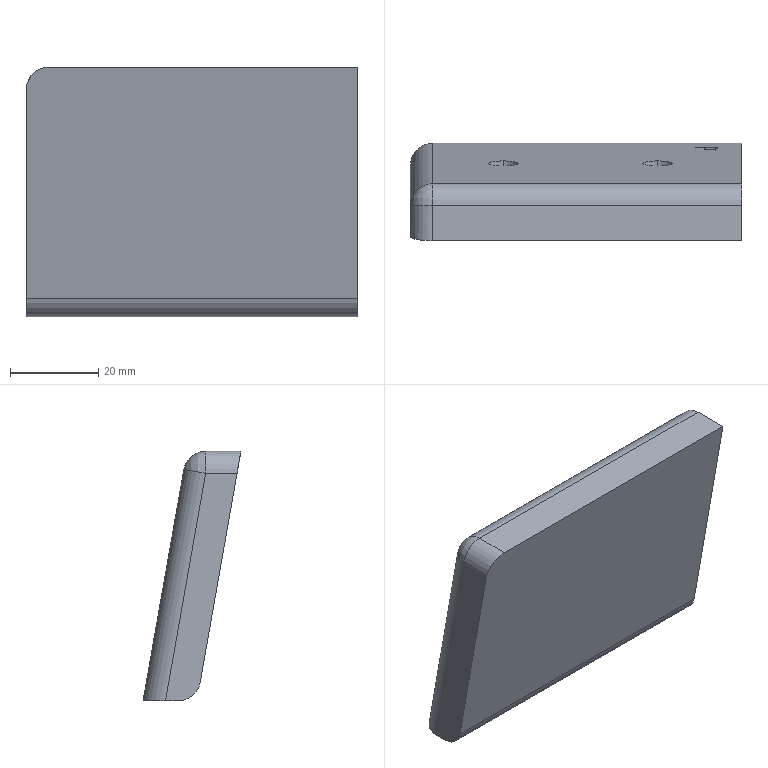Part | SolidWorks | features BaseBody 1 | 1 solid | 33 faces | box 75 x 22.148 x 56.5 mm | volume 50046 mm3 | plane 20 | cylinder 8 | cone 4 | sphere 1 | commonest cylinder face diameters 6.8 x4 10 x4
STEP:
#1=CARTESIAN_POINT('',(98.,284.297,22.336));
#2=VERTEX_POINT('',#1);
#3=CARTESIAN_POINT('',(98.,283.116,29.032));
#4=VERTEX_POINT('',#3);
#5=CARTESIAN_POINT('',(98.,283.707,25.684));
#6=DIRECTION('',(0.,0.9848,0.1736));
#7=DIRECTION('',(0.,0.1736,-0.9848));
#8=AXIS2_PLACEMENT_3D('',#5,#6,#7);
#9=CIRCLE('',#8,3.4);
#10=EDGE_CURVE('',#2,#4,#9,.T.);
#11=ORIENTED_EDGE('',*,*,#10,.T.);
#12=CARTESIAN_POINT('',(98.,274.253,27.47));
#13=VERTEX_POINT('',#12);
#14=CARTESIAN_POINT('',(98.,283.116,29.032));
#15=DIRECTION('',(0.,-0.9848,-0.1736));
#16=VECTOR('',#15,1000.);
#17=LINE('',#14,#16);
#18=EDGE_CURVE('',#4,#13,#17,.T.);
#19=ORIENTED_EDGE('',*,*,#18,.T.);
#20=CARTESIAN_POINT('',(98.,275.434,20.773));
#21=VERTEX_POINT('',#20);
#22=CARTESIAN_POINT('',(98.,274.843,24.121));
#23=DIRECTION('',(0.,0.9848,0.1736));
#24=DIRECTION('',(0.,0.1736,-0.9848));
#25=AXIS2_PLACEMENT_3D('',#22,#23,#24);
#26=CIRCLE('',#25,3.4);
#27=EDGE_CURVE('',#21,#13,#26,.T.);
#28=ORIENTED_EDGE('',*,*,#27,.F.);
#29=CARTESIAN_POINT('',(98.,284.297,22.336));
#30=DIRECTION('',(0.,-0.9848,-0.1736));
#31=VECTOR('',#30,1000.);
#32=LINE('',#29,#31);
#33=EDGE_CURVE('',#2,#21,#32,.T.);
#34=ORIENTED_EDGE('',*,*,#33,.F.);
#35=EDGE_LOOP('',(#11,#19,#28,#34));
#36=FACE_OUTER_BOUND('',#35,.T.);
#37=CARTESIAN_POINT('',(98.,283.707,25.684));
#38=DIRECTION('',(0.,-0.9848,-0.1736));
#39=DIRECTION('',(0.,0.1736,-0.9848));
#40=AXIS2_PLACEMENT_3D('',#37,#38,#39);
#41=CYLINDRICAL_SURFACE('',#40,3.4);
#42=ADVANCED_FACE('',(#36),#41,.F.);
#43=CARTESIAN_POINT('',(98.,272.831,23.767));
#44=VERTEX_POINT('',#43);
#45=CARTESIAN_POINT('',(98.,274.253,27.47));
#46=DIRECTION('',(0.,0.3584,0.9336));
#47=VECTOR('',#46,1000.);
#48=LINE('',#45,#47);
#49=EDGE_CURVE('',#44,#13,#48,.T.);
#50=ORIENTED_EDGE('',*,*,#49,.F.);
#51=CARTESIAN_POINT('',(98.,275.434,20.773));
#52=DIRECTION('',(0.,0.6561,-0.7547));
#53=VECTOR('',#52,1000.);
#54=LINE('',#51,#53);
#55=EDGE_CURVE('',#44,#21,#54,.T.);
#56=ORIENTED_EDGE('',*,*,#55,.T.);
#57=ORIENTED_EDGE('',*,*,#27,.T.);
#58=EDGE_LOOP('',(#50,#56,#57));
#59=FACE_OUTER_BOUND('',#58,.T.);
#60=CARTESIAN_POINT('',(98.,274.843,24.121));
#61=DIRECTION('',(0.,0.9848,0.1736));
#62=DIRECTION('',(0.,-0.1736,0.9848));
#63=AXIS2_PLACEMENT_3D('',#60,#61,#62);
#64=CONICAL_SURFACE('',#63,3.4,1.03);
#65=ADVANCED_FACE('',(#59),#64,.F.);
#66=CARTESIAN_POINT('',(133.,284.297,22.336));
#67=VERTEX_POINT('',#66);
#68=CARTESIAN_POINT('',(133.,283.116,29.032));
#69=VERTEX_POINT('',#68);
#70=CARTESIAN_POINT('',(133.,283.707,25.684));
#71=DIRECTION('',(0.,0.9848,0.1736));
#72=DIRECTION('',(0.,0.1736,-0.9848));
#73=AXIS2_PLACEMENT_3D('',#70,#71,#72);
#74=CIRCLE('',#73,3.4);
#75=EDGE_CURVE('',#67,#69,#74,.T.);
#76=ORIENTED_EDGE('',*,*,#75,.T.);
#77=CARTESIAN_POINT('',(133.,274.253,27.47));
#78=VERTEX_POINT('',#77);
#79=CARTESIAN_POINT('',(133.,283.116,29.032));
#80=DIRECTION('',(0.,-0.9848,-0.1736));
#81=VECTOR('',#80,1000.);
#82=LINE('',#79,#81);
#83=EDGE_CURVE('',#69,#78,#82,.T.);
#84=ORIENTED_EDGE('',*,*,#83,.T.);
#85=CARTESIAN_POINT('',(133.,275.434,20.773));
#86=VERTEX_POINT('',#85);
#87=CARTESIAN_POINT('',(133.,274.843,24.121));
#88=DIRECTION('',(0.,0.9848,0.1736));
#89=DIRECTION('',(0.,0.1736,-0.9848));
#90=AXIS2_PLACEMENT_3D('',#87,#88,#89);
#91=CIRCLE('',#90,3.4);
#92=EDGE_CURVE('',#86,#78,#91,.T.);
#93=ORIENTED_EDGE('',*,*,#92,.F.);
#94=CARTESIAN_POINT('',(133.,284.297,22.336));
#95=DIRECTION('',(0.,-0.9848,-0.1736));
#96=VECTOR('',#95,1000.);
#97=LINE('',#94,#96);
#98=EDGE_CURVE('',#67,#86,#97,.T.);
#99=ORIENTED_EDGE('',*,*,#98,.F.);
#100=EDGE_LOOP('',(#76,#84,#93,#99));
#101=FACE_OUTER_BOUND('',#100,.T.);
#102=CARTESIAN_POINT('',(133.,283.707,25.684));
#103=DIRECTION('',(0.,-0.9848,-0.1736));
#104=DIRECTION('',(0.,0.1736,-0.9848));
#105=AXIS2_PLACEMENT_3D('',#102,#103,#104);
#106=CYLINDRICAL_SURFACE('',#105,3.4);
#107=ADVANCED_FACE('',(#101),#106,.F.);
#108=CARTESIAN_POINT('',(133.,272.831,23.767));
#109=VERTEX_POINT('',#108);
#110=CARTESIAN_POINT('',(133.,274.253,27.47));
#111=DIRECTION('',(0.,0.3584,0.9336));
#112=VECTOR('',#111,1000.);
#113=LINE('',#110,#112);
#114=EDGE_CURVE('',#109,#78,#113,.T.);
#115=ORIENTED_EDGE('',*,*,#114,.F.);
#116=CARTESIAN_POINT('',(133.,275.434,20.773));
#117=DIRECTION('',(0.,0.6561,-0.7547));
#118=VECTOR('',#117,1000.);
#119=LINE('',#116,#118);
#120=EDGE_CURVE('',#109,#86,#119,.T.);
#121=ORIENTED_EDGE('',*,*,#120,.T.);
#122=ORIENTED_EDGE('',*,*,#92,.T.);
#123=EDGE_LOOP('',(#115,#121,#122));
#124=FACE_OUTER_BOUND('',#123,.T.);
#125=CARTESIAN_POINT('',(133.,274.843,24.121));
#126=DIRECTION('',(0.,0.9848,0.1736));
#127=DIRECTION('',(0.,-0.1736,0.9848));
#128=AXIS2_PLACEMENT_3D('',#125,#126,#127);
#129=CONICAL_SURFACE('',#128,3.4,1.03);
#130=ADVANCED_FACE('',(#124),#129,.F.);
#131=CARTESIAN_POINT('',(77.,267.058,51.));
#132=VERTEX_POINT('',#131);
#133=CARTESIAN_POINT('',(77.,275.41,3.632));
#134=VERTEX_POINT('',#133);
#135=CARTESIAN_POINT('',(77.,270.574,31.056));
#136=DIRECTION('',(0.,0.1736,-0.9848));
#137=VECTOR('',#136,1000.);
#138=LINE('',#135,#137);
#139=EDGE_CURVE('',#132,#134,#138,.T.);
#140=ORIENTED_EDGE('',*,*,#139,.T.);
#141=CARTESIAN_POINT('',(152.,275.41,3.632));
#142=VERTEX_POINT('',#141);
#143=CARTESIAN_POINT('',(-4.,275.41,3.632));
#144=DIRECTION('',(-1.,0.,0.));
#145=VECTOR('',#144,1000.);
#146=LINE('',#143,#145);
#147=EDGE_CURVE('',#142,#134,#146,.T.);
#148=ORIENTED_EDGE('',*,*,#147,.F.);
#149=CARTESIAN_POINT('',(152.,266.176,56.));
#150=VERTEX_POINT('',#149);
#151=CARTESIAN_POINT('',(152.,271.705,24.642));
#152=DIRECTION('',(0.,0.1736,-0.9848));
#153=VECTOR('',#152,1000.);
#154=LINE('',#151,#153);
#155=EDGE_CURVE('',#150,#142,#154,.T.);
#156=ORIENTED_EDGE('',*,*,#155,.F.);
#157=CARTESIAN_POINT('',(82.,266.176,56.));
#158=VERTEX_POINT('',#157);
#159=CARTESIAN_POINT('',(-4.,266.176,56.));
#160=DIRECTION('',(-1.,0.,0.));
#161=VECTOR('',#160,1000.);
#162=LINE('',#159,#161);
#163=EDGE_CURVE('',#150,#158,#162,.T.);
#164=ORIENTED_EDGE('',*,*,#163,.T.);
#165=CARTESIAN_POINT('',(77.,267.058,51.));
#166=CARTESIAN_POINT('',(77.,266.541,53.929));
#167=CARTESIAN_POINT('',(79.071,266.176,56.));
#168=CARTESIAN_POINT('',(82.,266.176,56.));
#169=(BOUNDED_CURVE()B_SPLINE_CURVE(3,(#165,#166,#167,#168),.UNSPECIFIED.,.F.,.T.)B_SPLINE_CURVE_WITH_KNOTS((4,4),(4.712,6.283),.UNSPECIFIED.)CURVE()GEOMETRIC_REPRESENTATION_ITEM()RATIONAL_B_SPLINE_CURVE((1.,0.8047,0.8047,1.))REPRESENTATION_ITEM(''));
#170=EDGE_CURVE('',#132,#158,#169,.T.);
#171=ORIENTED_EDGE('',*,*,#170,.F.);
#172=EDGE_LOOP('',(#140,#148,#156,#164,#171));
#173=FACE_OUTER_BOUND('',#172,.T.);
#174=CARTESIAN_POINT('',(-4.,266.352,55.));
#175=DIRECTION('',(0.,0.9848,0.1736));
#176=DIRECTION('',(0.,-0.1736,0.9848));
#177=AXIS2_PLACEMENT_3D('',#174,#175,#176);
#178=PLANE('',#177);
#179=ADVANCED_FACE('',(#173),#178,.F.);
#180=CARTESIAN_POINT('',(146.015,286.85,7.856));
#181=VERTEX_POINT('',#180);
#182=CARTESIAN_POINT('',(146.015,286.503,9.826));
#183=VERTEX_POINT('',#182);
#184=CARTESIAN_POINT('',(146.015,286.85,7.856));
#185=DIRECTION('',(0.,-0.1736,0.9848));
#186=VECTOR('',#185,1000.);
#187=LINE('',#184,#186);
#188=EDGE_CURVE('',#181,#183,#187,.T.);
#189=ORIENTED_EDGE('',*,*,#188,.F.);
#190=CARTESIAN_POINT('',(143.515,286.85,7.856));
#191=VERTEX_POINT('',#190);
#192=CARTESIAN_POINT('',(146.015,286.85,7.856));
#193=DIRECTION('',(-1.,0.,0.));
#194=VECTOR('',#193,1000.);
#195=LINE('',#192,#194);
#196=EDGE_CURVE('',#181,#191,#195,.T.);
#197=ORIENTED_EDGE('',*,*,#196,.T.);
#198=CARTESIAN_POINT('',(143.515,287.284,5.394));
#199=VERTEX_POINT('',#198);
#200=CARTESIAN_POINT('',(143.515,287.284,5.394));
#201=DIRECTION('',(0.,-0.1736,0.9848));
#202=VECTOR('',#201,1000.);
#203=LINE('',#200,#202);
#204=EDGE_CURVE('',#199,#191,#203,.T.);
#205=ORIENTED_EDGE('',*,*,#204,.F.);
#206=CARTESIAN_POINT('',(141.515,287.284,5.394));
#207=VERTEX_POINT('',#206);
#208=CARTESIAN_POINT('',(143.515,287.284,5.394));
#209=DIRECTION('',(-1.,0.,0.));
#210=VECTOR('',#209,1000.);
#211=LINE('',#208,#210);
#212=EDGE_CURVE('',#199,#207,#211,.T.);
#213=ORIENTED_EDGE('',*,*,#212,.T.);
#214=CARTESIAN_POINT('',(141.515,287.371,4.902));
#215=VERTEX_POINT('',#214);
#216=CARTESIAN_POINT('',(141.515,287.284,5.394));
#217=DIRECTION('',(0.,0.1736,-0.9848));
#218=VECTOR('',#217,1000.);
#219=LINE('',#216,#218);
#220=EDGE_CURVE('',#207,#215,#219,.T.);
#221=ORIENTED_EDGE('',*,*,#220,.T.);
#222=CARTESIAN_POINT('',(146.515,287.371,4.902));
#223=VERTEX_POINT('',#222);
#224=CARTESIAN_POINT('',(146.515,287.371,4.902));
#225=DIRECTION('',(-1.,0.,0.));
#226=VECTOR('',#225,1000.);
#227=LINE('',#224,#226);
#228=EDGE_CURVE('',#223,#215,#227,.T.);
#229=ORIENTED_EDGE('',*,*,#228,.F.);
#230=CARTESIAN_POINT('',(146.515,286.503,9.826));
#231=VERTEX_POINT('',#230);
#232=CARTESIAN_POINT('',(146.515,287.371,4.902));
#233=DIRECTION('',(0.,-0.1736,0.9848));
#234=VECTOR('',#233,1000.);
#235=LINE('',#232,#234);
#236=EDGE_CURVE('',#223,#231,#235,.T.);
#237=ORIENTED_EDGE('',*,*,#236,.T.);
#238=CARTESIAN_POINT('',(146.515,286.503,9.826));
#239=DIRECTION('',(-1.,0.,0.));
#240=VECTOR('',#239,1000.);
#241=LINE('',#238,#240);
#242=EDGE_CURVE('',#231,#183,#241,.T.);
#243=ORIENTED_EDGE('',*,*,#242,.T.);
#244=EDGE_LOOP('',(#189,#197,#205,#213,#221,#229,#237,#243));
#245=FACE_BOUND('',#244,.T.);
#246=ORIENTED_EDGE('',*,*,#75,.F.);
#247=CARTESIAN_POINT('',(133.,283.707,25.684));
#248=DIRECTION('',(0.,0.9848,0.1736));
#249=DIRECTION('',(0.,0.1736,-0.9848));
#250=AXIS2_PLACEMENT_3D('',#247,#248,#249);
#251=CIRCLE('',#250,3.4);
#252=EDGE_CURVE('',#69,#67,#251,.T.);
#253=ORIENTED_EDGE('',*,*,#252,.F.);
#254=EDGE_LOOP('',(#246,#253));
#255=FACE_BOUND('',#254,.T.);
#256=ORIENTED_EDGE('',*,*,#10,.F.);
#257=CARTESIAN_POINT('',(98.,283.707,25.684));
#258=DIRECTION('',(0.,0.9848,0.1736));
#259=DIRECTION('',(0.,0.1736,-0.9848));
#260=AXIS2_PLACEMENT_3D('',#257,#258,#259);
#261=CIRCLE('',#260,3.4);
#262=EDGE_CURVE('',#4,#2,#261,.T.);
#263=ORIENTED_EDGE('',*,*,#262,.F.);
#264=EDGE_LOOP('',(#256,#263));
#265=FACE_BOUND('',#264,.T.);
#266=CARTESIAN_POINT('',(82.,279.09,51.868));
#267=VERTEX_POINT('',#266);
#268=CARTESIAN_POINT('',(152.,279.09,51.868));
#269=VERTEX_POINT('',#268);
#270=CARTESIAN_POINT('',(188.,279.09,51.868));
#271=DIRECTION('',(1.,0.,0.));
#272=VECTOR('',#271,1000.);
#273=LINE('',#270,#272);
#274=EDGE_CURVE('',#267,#269,#273,.T.);
#275=ORIENTED_EDGE('',*,*,#274,.T.);
#276=CARTESIAN_POINT('',(152.,288.324,-0.5));
#277=VERTEX_POINT('',#276);
#278=CARTESIAN_POINT('',(152.,283.523,26.726));
#279=DIRECTION('',(0.,0.1736,-0.9848));
#280=VECTOR('',#279,1000.);
#281=LINE('',#278,#280);
#282=EDGE_CURVE('',#269,#277,#281,.T.);
#283=ORIENTED_EDGE('',*,*,#282,.T.);
#284=CARTESIAN_POINT('',(82.,288.324,-0.5));
#285=VERTEX_POINT('',#284);
#286=CARTESIAN_POINT('',(-429.,288.324,-0.5));
#287=DIRECTION('',(1.,0.,0.));
#288=VECTOR('',#287,1000.);
#289=LINE('',#286,#288);
#290=EDGE_CURVE('',#285,#277,#289,.T.);
#291=ORIENTED_EDGE('',*,*,#290,.F.);
#292=CARTESIAN_POINT('',(82.,288.324,-0.5));
#293=DIRECTION('',(0.,0.1736,-0.9848));
#294=VECTOR('',#293,1000.);
#295=LINE('',#292,#294);
#296=EDGE_CURVE('',#267,#285,#295,.T.);
#297=ORIENTED_EDGE('',*,*,#296,.F.);
#298=EDGE_LOOP('',(#275,#283,#291,#297));
#299=FACE_OUTER_BOUND('',#298,.T.);
#300=CARTESIAN_POINT('',(140.5,282.887,30.334));
#301=DIRECTION('',(0.,-0.9848,-0.1736));
#302=DIRECTION('',(0.,0.1736,-0.9848));
#303=AXIS2_PLACEMENT_3D('',#300,#301,#302);
#304=PLANE('',#303);
#305=ADVANCED_FACE('',(#245,#255,#265,#299),#304,.F.);
#306=ORIENTED_EDGE('',*,*,#163,.F.);
#307=CARTESIAN_POINT('',(152.,274.166,56.));
#308=VERTEX_POINT('',#307);
#309=CARTESIAN_POINT('',(152.,275.152,56.));
#310=DIRECTION('',(0.,1.,0.));
#311=VECTOR('',#310,1000.);
#312=LINE('',#309,#311);
#313=EDGE_CURVE('',#150,#308,#312,.T.);
#314=ORIENTED_EDGE('',*,*,#313,.T.);
#315=CARTESIAN_POINT('',(82.,274.166,56.));
#316=VERTEX_POINT('',#315);
#317=CARTESIAN_POINT('',(93.,274.166,56.));
#318=DIRECTION('',(-1.,0.,0.));
#319=VECTOR('',#318,1000.);
#320=LINE('',#317,#319);
#321=EDGE_CURVE('',#308,#316,#320,.T.);
#322=ORIENTED_EDGE('',*,*,#321,.T.);
#323=CARTESIAN_POINT('',(82.,274.166,56.));
#324=DIRECTION('',(0.,1.,0.));
#325=VECTOR('',#324,1000.);
#326=LINE('',#323,#325);
#327=EDGE_CURVE('',#158,#316,#326,.T.);
#328=ORIENTED_EDGE('',*,*,#327,.F.);
#329=EDGE_LOOP('',(#306,#314,#322,#328));
#330=FACE_OUTER_BOUND('',#329,.T.);
#331=CARTESIAN_POINT('',(138.,235.588,56.));
#332=DIRECTION('',(0.,0.,-1.));
#333=DIRECTION('',(1.,0.,0.));
#334=AXIS2_PLACEMENT_3D('',#331,#332,#333);
#335=PLANE('',#334);
#336=ADVANCED_FACE('',(#330),#335,.F.);
#337=ORIENTED_EDGE('',*,*,#290,.T.);
#338=CARTESIAN_POINT('',(152.,280.334,-0.5));
#339=VERTEX_POINT('',#338);
#340=CARTESIAN_POINT('',(152.,275.152,-0.5));
#341=DIRECTION('',(0.,1.,0.));
#342=VECTOR('',#341,1000.);
#343=LINE('',#340,#342);
#344=EDGE_CURVE('',#339,#277,#343,.T.);
#345=ORIENTED_EDGE('',*,*,#344,.F.);
#346=CARTESIAN_POINT('',(77.,280.334,-0.5));
#347=VERTEX_POINT('',#346);
#348=CARTESIAN_POINT('',(-429.,280.334,-0.5));
#349=DIRECTION('',(1.,0.,0.));
#350=VECTOR('',#349,1000.);
#351=LINE('',#348,#350);
#352=EDGE_CURVE('',#347,#339,#351,.T.);
#353=ORIENTED_EDGE('',*,*,#352,.F.);
#354=CARTESIAN_POINT('',(77.,283.246,-0.5));
#355=VERTEX_POINT('',#354);
#356=CARTESIAN_POINT('',(77.,355.,-0.5));
#357=DIRECTION('',(0.,-1.,0.));
#358=VECTOR('',#357,1000.);
#359=LINE('',#356,#358);
#360=EDGE_CURVE('',#355,#347,#359,.T.);
#361=ORIENTED_EDGE('',*,*,#360,.F.);
#362=CARTESIAN_POINT('',(82.,288.324,-0.5));
#363=CARTESIAN_POINT('',(79.071,288.324,-0.5));
#364=CARTESIAN_POINT('',(77.,286.221,-0.5));
#365=CARTESIAN_POINT('',(77.,283.246,-0.5));
#366=(BOUNDED_CURVE()B_SPLINE_CURVE(3,(#362,#363,#364,#365),.UNSPECIFIED.,.F.,.T.)B_SPLINE_CURVE_WITH_KNOTS((4,4),(0.,1.571),.UNSPECIFIED.)CURVE()GEOMETRIC_REPRESENTATION_ITEM()RATIONAL_B_SPLINE_CURVE((1.,0.8047,0.8047,1.))REPRESENTATION_ITEM(''));
#367=EDGE_CURVE('',#285,#355,#366,.T.);
#368=ORIENTED_EDGE('',*,*,#367,.F.);
#369=EDGE_LOOP('',(#337,#345,#353,#361,#368));
#370=FACE_OUTER_BOUND('',#369,.T.);
#371=CARTESIAN_POINT('',(-429.,355.,-0.5));
#372=DIRECTION('',(0.,0.,-1.));
#373=DIRECTION('',(1.,0.,0.));
#374=AXIS2_PLACEMENT_3D('',#371,#372,#373);
#375=PLANE('',#374);
#376=ADVANCED_FACE('',(#370),#375,.T.);
#377=ORIENTED_EDGE('',*,*,#321,.F.);
#378=CARTESIAN_POINT('',(152.,274.166,51.));
#379=DIRECTION('',(1.,0.,0.));
#380=DIRECTION('',(0.,0.,-1.));
#381=AXIS2_PLACEMENT_3D('',#378,#379,#380);
#382=CIRCLE('',#381,5.);
#383=EDGE_CURVE('',#269,#308,#382,.T.);
#384=ORIENTED_EDGE('',*,*,#383,.F.);
#385=ORIENTED_EDGE('',*,*,#274,.F.);
#386=CARTESIAN_POINT('',(82.,274.166,51.));
#387=DIRECTION('',(-1.,0.,0.));
#388=DIRECTION('',(0.,1.,0.));
#389=AXIS2_PLACEMENT_3D('',#386,#387,#388);
#390=CIRCLE('',#389,5.);
#391=EDGE_CURVE('',#316,#267,#390,.T.);
#392=ORIENTED_EDGE('',*,*,#391,.F.);
#393=EDGE_LOOP('',(#377,#384,#385,#392));
#394=FACE_OUTER_BOUND('',#393,.T.);
#395=CARTESIAN_POINT('',(140.5,274.166,51.));
#396=DIRECTION('',(-1.,0.,0.));
#397=DIRECTION('',(0.,1.,0.));
#398=AXIS2_PLACEMENT_3D('',#395,#396,#397);
#399=CYLINDRICAL_SURFACE('',#398,5.);
#400=ADVANCED_FACE('',(#394),#399,.T.);
#401=ORIENTED_EDGE('',*,*,#147,.T.);
#402=CARTESIAN_POINT('',(77.,280.334,4.5));
#403=DIRECTION('',(1.,0.,0.));
#404=DIRECTION('',(0.,0.,-1.));
#405=AXIS2_PLACEMENT_3D('',#402,#403,#404);
#406=CIRCLE('',#405,5.);
#407=EDGE_CURVE('',#134,#347,#406,.T.);
#408=ORIENTED_EDGE('',*,*,#407,.T.);
#409=ORIENTED_EDGE('',*,*,#352,.T.);
#410=CARTESIAN_POINT('',(152.,280.334,4.5));
#411=DIRECTION('',(1.,0.,0.));
#412=DIRECTION('',(0.,0.,-1.));
#413=AXIS2_PLACEMENT_3D('',#410,#411,#412);
#414=CIRCLE('',#413,5.);
#415=EDGE_CURVE('',#142,#339,#414,.T.);
#416=ORIENTED_EDGE('',*,*,#415,.F.);
#417=EDGE_LOOP('',(#401,#408,#409,#416));
#418=FACE_OUTER_BOUND('',#417,.T.);
#419=CARTESIAN_POINT('',(-4.,280.334,4.5));
#420=DIRECTION('',(1.,0.,0.));
#421=DIRECTION('',(0.,-1.,0.));
#422=AXIS2_PLACEMENT_3D('',#419,#420,#421);
#423=CYLINDRICAL_SURFACE('',#422,5.);
#424=ADVANCED_FACE('',(#418),#423,.T.);
#425=CARTESIAN_POINT('',(77.,274.166,51.));
#426=VERTEX_POINT('',#425);
#427=CARTESIAN_POINT('',(77.,274.166,51.));
#428=DIRECTION('',(0.,-0.1736,0.9848));
#429=VECTOR('',#428,1000.);
#430=LINE('',#427,#429);
#431=EDGE_CURVE('',#355,#426,#430,.T.);
#432=ORIENTED_EDGE('',*,*,#431,.F.);
#433=ORIENTED_EDGE('',*,*,#360,.T.);
#434=ORIENTED_EDGE('',*,*,#407,.F.);
#435=ORIENTED_EDGE('',*,*,#139,.F.);
#436=CARTESIAN_POINT('',(77.,266.176,51.));
#437=DIRECTION('',(0.,-1.,0.));
#438=VECTOR('',#437,1000.);
#439=LINE('',#436,#438);
#440=EDGE_CURVE('',#426,#132,#439,.T.);
#441=ORIENTED_EDGE('',*,*,#440,.F.);
#442=EDGE_LOOP('',(#432,#433,#434,#435,#441));
#443=FACE_OUTER_BOUND('',#442,.T.);
#444=CARTESIAN_POINT('',(77.,240.481,25.75));
#445=DIRECTION('',(-1.,0.,0.));
#446=DIRECTION('',(0.,0.,-1.));
#447=AXIS2_PLACEMENT_3D('',#444,#445,#446);
#448=PLANE('',#447);
#449=ADVANCED_FACE('',(#443),#448,.T.);
#450=ORIENTED_EDGE('',*,*,#120,.F.);
#451=ORIENTED_EDGE('',*,*,#114,.T.);
#452=CARTESIAN_POINT('',(133.,274.843,24.121));
#453=DIRECTION('',(0.,0.9848,0.1736));
#454=DIRECTION('',(0.,0.1736,-0.9848));
#455=AXIS2_PLACEMENT_3D('',#452,#453,#454);
#456=CIRCLE('',#455,3.4);
#457=EDGE_CURVE('',#78,#86,#456,.T.);
#458=ORIENTED_EDGE('',*,*,#457,.T.);
#459=EDGE_LOOP('',(#450,#451,#458));
#460=FACE_OUTER_BOUND('',#459,.T.);
#461=CARTESIAN_POINT('',(133.,274.843,24.121));
#462=DIRECTION('',(0.,0.9848,0.1736));
#463=DIRECTION('',(0.,-0.1736,0.9848));
#464=AXIS2_PLACEMENT_3D('',#461,#462,#463);
#465=CONICAL_SURFACE('',#464,3.4,1.03);
#466=ADVANCED_FACE('',(#460),#465,.F.);
#467=ORIENTED_EDGE('',*,*,#83,.F.);
#468=ORIENTED_EDGE('',*,*,#252,.T.);
#469=ORIENTED_EDGE('',*,*,#98,.T.);
#470=ORIENTED_EDGE('',*,*,#457,.F.);
#471=EDGE_LOOP('',(#467,#468,#469,#470));
#472=FACE_OUTER_BOUND('',#471,.T.);
#473=CARTESIAN_POINT('',(133.,283.707,25.684));
#474=DIRECTION('',(0.,-0.9848,-0.1736));
#475=DIRECTION('',(0.,0.1736,-0.9848));
#476=AXIS2_PLACEMENT_3D('',#473,#474,#475);
#477=CYLINDRICAL_SURFACE('',#476,3.4);
#478=ADVANCED_FACE('',(#472),#477,.F.);
#479=ORIENTED_EDGE('',*,*,#55,.F.);
#480=ORIENTED_EDGE('',*,*,#49,.T.);
#481=CARTESIAN_POINT('',(98.,274.843,24.121));
#482=DIRECTION('',(0.,0.9848,0.1736));
#483=DIRECTION('',(0.,0.1736,-0.9848));
#484=AXIS2_PLACEMENT_3D('',#481,#482,#483);
#485=CIRCLE('',#484,3.4);
#486=EDGE_CURVE('',#13,#21,#485,.T.);
#487=ORIENTED_EDGE('',*,*,#486,.T.);
#488=EDGE_LOOP('',(#479,#480,#487));
#489=FACE_OUTER_BOUND('',#488,.T.);
#490=CARTESIAN_POINT('',(98.,274.843,24.121));
#491=DIRECTION('',(0.,0.9848,0.1736));
#492=DIRECTION('',(0.,-0.1736,0.9848));
#493=AXIS2_PLACEMENT_3D('',#490,#491,#492);
#494=CONICAL_SURFACE('',#493,3.4,1.03);
#495=ADVANCED_FACE('',(#489),#494,.F.);
#496=ORIENTED_EDGE('',*,*,#18,.F.);
#497=ORIENTED_EDGE('',*,*,#262,.T.);
#498=ORIENTED_EDGE('',*,*,#33,.T.);
#499=ORIENTED_EDGE('',*,*,#486,.F.);
#500=EDGE_LOOP('',(#496,#497,#498,#499));
#501=FACE_OUTER_BOUND('',#500,.T.);
#502=CARTESIAN_POINT('',(98.,283.707,25.684));
#503=DIRECTION('',(0.,-0.9848,-0.1736));
#504=DIRECTION('',(0.,0.1736,-0.9848));
#505=AXIS2_PLACEMENT_3D('',#502,#503,#504);
#506=CYLINDRICAL_SURFACE('',#505,3.4);
#507=ADVANCED_FACE('',(#501),#506,.F.);
#508=ORIENTED_EDGE('',*,*,#155,.T.);
#509=ORIENTED_EDGE('',*,*,#415,.T.);
#510=ORIENTED_EDGE('',*,*,#344,.T.);
#511=ORIENTED_EDGE('',*,*,#282,.F.);
#512=ORIENTED_EDGE('',*,*,#383,.T.);
#513=ORIENTED_EDGE('',*,*,#313,.F.);
#514=EDGE_LOOP('',(#508,#509,#510,#511,#512,#513));
#515=FACE_OUTER_BOUND('',#514,.T.);
#516=CARTESIAN_POINT('',(152.,275.152,25.25));
#517=DIRECTION('',(1.,0.,0.));
#518=DIRECTION('',(0.,0.,1.));
#519=AXIS2_PLACEMENT_3D('',#516,#517,#518);
#520=PLANE('',#519);
#521=ADVANCED_FACE('',(#515),#520,.T.);
#522=ORIENTED_EDGE('',*,*,#367,.T.);
#523=ORIENTED_EDGE('',*,*,#431,.T.);
#524=CARTESIAN_POINT('',(82.,274.166,51.));
#525=DIRECTION('',(0.,0.1736,-0.9848));
#526=DIRECTION('',(0.,-0.9848,-0.1736));
#527=AXIS2_PLACEMENT_3D('',#524,#525,#526);
#528=CIRCLE('',#527,5.);
#529=EDGE_CURVE('',#426,#267,#528,.T.);
#530=ORIENTED_EDGE('',*,*,#529,.T.);
#531=ORIENTED_EDGE('',*,*,#296,.T.);
#532=EDGE_LOOP('',(#522,#523,#530,#531));
#533=FACE_OUTER_BOUND('',#532,.T.);
#534=CARTESIAN_POINT('',(82.,277.468,32.272));
#535=DIRECTION('',(0.,0.1736,-0.9848));
#536=DIRECTION('',(0.,0.9848,0.1736));
#537=AXIS2_PLACEMENT_3D('',#534,#535,#536);
#538=CYLINDRICAL_SURFACE('',#537,5.);
#539=ADVANCED_FACE('',(#533),#538,.T.);
#540=ORIENTED_EDGE('',*,*,#529,.F.);
#541=CARTESIAN_POINT('',(82.,274.166,51.));
#542=DIRECTION('',(0.,1.,0.));
#543=DIRECTION('',(0.,0.,-1.));
#544=AXIS2_PLACEMENT_3D('',#541,#542,#543);
#545=CIRCLE('',#544,5.);
#546=EDGE_CURVE('',#426,#316,#545,.T.);
#547=ORIENTED_EDGE('',*,*,#546,.T.);
#548=ORIENTED_EDGE('',*,*,#391,.T.);
#549=EDGE_LOOP('',(#540,#547,#548));
#550=FACE_OUTER_BOUND('',#549,.T.);
#551=CARTESIAN_POINT('',(82.,274.166,51.));
#552=DIRECTION('',(0.,-1.,0.));
#553=DIRECTION('',(-1.,0.,0.));
#554=AXIS2_PLACEMENT_3D('',#551,#552,#553);
#555=SPHERICAL_SURFACE('',#554,5.);
#556=ADVANCED_FACE('',(#550),#555,.T.);
#557=ORIENTED_EDGE('',*,*,#170,.T.);
#558=ORIENTED_EDGE('',*,*,#327,.T.);
#559=ORIENTED_EDGE('',*,*,#546,.F.);
#560=ORIENTED_EDGE('',*,*,#440,.T.);
#561=EDGE_LOOP('',(#557,#558,#559,#560));
#562=FACE_OUTER_BOUND('',#561,.T.);
#563=CARTESIAN_POINT('',(82.,235.588,51.));
#564=DIRECTION('',(0.,-1.,0.));
#565=DIRECTION('',(0.,0.,-1.));
#566=AXIS2_PLACEMENT_3D('',#563,#564,#565);
#567=CYLINDRICAL_SURFACE('',#566,5.);
#568=ADVANCED_FACE('',(#562),#567,.T.);
#569=CARTESIAN_POINT('',(146.015,287.038,5.351));
#570=VERTEX_POINT('',#569);
#571=CARTESIAN_POINT('',(146.015,286.691,7.32));
#572=VERTEX_POINT('',#571);
#573=CARTESIAN_POINT('',(146.015,287.038,5.351));
#574=DIRECTION('',(0.,-0.1736,0.9848));
#575=VECTOR('',#574,1000.);
#576=LINE('',#573,#575);
#577=EDGE_CURVE('',#570,#572,#576,.T.);
#578=ORIENTED_EDGE('',*,*,#577,.F.);
#579=CARTESIAN_POINT('',(146.015,287.284,5.394));
#580=VERTEX_POINT('',#579);
#581=CARTESIAN_POINT('',(146.015,287.284,5.394));
#582=DIRECTION('',(0.,-0.9848,-0.1736));
#583=VECTOR('',#582,1000.);
#584=LINE('',#581,#583);
#585=EDGE_CURVE('',#580,#570,#584,.T.);
#586=ORIENTED_EDGE('',*,*,#585,.F.);
#587=CARTESIAN_POINT('',(146.015,286.937,7.364));
#588=VERTEX_POINT('',#587);
#589=CARTESIAN_POINT('',(146.015,287.284,5.394));
#590=DIRECTION('',(0.,-0.1736,0.9848));
#591=VECTOR('',#590,1000.);
#592=LINE('',#589,#591);
#593=EDGE_CURVE('',#580,#588,#592,.T.);
#594=ORIENTED_EDGE('',*,*,#593,.T.);
#595=CARTESIAN_POINT('',(146.015,286.937,7.364));
#596=DIRECTION('',(0.,-0.9848,-0.1736));
#597=VECTOR('',#596,1000.);
#598=LINE('',#595,#597);
#599=EDGE_CURVE('',#588,#572,#598,.T.);
#600=ORIENTED_EDGE('',*,*,#599,.T.);
#601=EDGE_LOOP('',(#578,#586,#594,#600));
#602=FACE_OUTER_BOUND('',#601,.T.);
#603=CARTESIAN_POINT('',(146.015,287.284,5.394));
#604=DIRECTION('',(1.,0.,0.));
#605=DIRECTION('',(0.,0.9848,0.1736));
#606=AXIS2_PLACEMENT_3D('',#603,#604,#605);
#607=PLANE('',#606);
#608=ADVANCED_FACE('',(#602),#607,.T.);
#609=CARTESIAN_POINT('',(144.015,287.038,5.351));
#610=VERTEX_POINT('',#609);
#611=CARTESIAN_POINT('',(146.015,287.038,5.351));
#612=DIRECTION('',(-1.,0.,0.));
#613=VECTOR('',#612,1000.);
#614=LINE('',#611,#613);
#615=EDGE_CURVE('',#570,#610,#614,.T.);
#616=ORIENTED_EDGE('',*,*,#615,.T.);
#617=CARTESIAN_POINT('',(144.015,287.284,5.394));
#618=VERTEX_POINT('',#617);
#619=CARTESIAN_POINT('',(144.015,287.284,5.394));
#620=DIRECTION('',(0.,-0.9848,-0.1736));
#621=VECTOR('',#620,1000.);
#622=LINE('',#619,#621);
#623=EDGE_CURVE('',#618,#610,#622,.T.);
#624=ORIENTED_EDGE('',*,*,#623,.F.);
#625=CARTESIAN_POINT('',(146.015,287.284,5.394));
#626=DIRECTION('',(-1.,0.,0.));
#627=VECTOR('',#626,1000.);
#628=LINE('',#625,#627);
#629=EDGE_CURVE('',#580,#618,#628,.T.);
#630=ORIENTED_EDGE('',*,*,#629,.F.);
#631=ORIENTED_EDGE('',*,*,#585,.T.);
#632=EDGE_LOOP('',(#616,#624,#630,#631));
#633=FACE_OUTER_BOUND('',#632,.T.);
#634=CARTESIAN_POINT('',(146.015,287.284,5.394));
#635=DIRECTION('',(0.,-0.1736,0.9848));
#636=DIRECTION('',(0.,0.9848,0.1736));
#637=AXIS2_PLACEMENT_3D('',#634,#635,#636);
#638=PLANE('',#637);
#639=ADVANCED_FACE('',(#633),#638,.F.);
#640=CARTESIAN_POINT('',(144.015,286.691,7.32));
#641=VERTEX_POINT('',#640);
#642=CARTESIAN_POINT('',(144.015,287.038,5.351));
#643=DIRECTION('',(0.,-0.1736,0.9848));
#644=VECTOR('',#643,1000.);
#645=LINE('',#642,#644);
#646=EDGE_CURVE('',#610,#641,#645,.T.);
#647=ORIENTED_EDGE('',*,*,#646,.T.);
#648=CARTESIAN_POINT('',(144.015,286.937,7.364));
#649=VERTEX_POINT('',#648);
#650=CARTESIAN_POINT('',(144.015,286.937,7.364));
#651=DIRECTION('',(0.,-0.9848,-0.1736));
#652=VECTOR('',#651,1000.);
#653=LINE('',#650,#652);
#654=EDGE_CURVE('',#649,#641,#653,.T.);
#655=ORIENTED_EDGE('',*,*,#654,.F.);
#656=CARTESIAN_POINT('',(144.015,287.284,5.394));
#657=DIRECTION('',(0.,-0.1736,0.9848));
#658=VECTOR('',#657,1000.);
#659=LINE('',#656,#658);
#660=EDGE_CURVE('',#618,#649,#659,.T.);
#661=ORIENTED_EDGE('',*,*,#660,.F.);
#662=ORIENTED_EDGE('',*,*,#623,.T.);
#663=EDGE_LOOP('',(#647,#655,#661,#662));
#664=FACE_OUTER_BOUND('',#663,.T.);
#665=CARTESIAN_POINT('',(144.015,287.284,5.394));
#666=DIRECTION('',(1.,0.,0.));
#667=DIRECTION('',(0.,0.9848,0.1736));
#668=AXIS2_PLACEMENT_3D('',#665,#666,#667);
#669=PLANE('',#668);
#670=ADVANCED_FACE('',(#664),#669,.F.);
#671=CARTESIAN_POINT('',(146.015,286.604,7.813));
#672=VERTEX_POINT('',#671);
#673=CARTESIAN_POINT('',(143.515,286.604,7.813));
#674=VERTEX_POINT('',#673);
#675=CARTESIAN_POINT('',(146.015,286.604,7.813));
#676=DIRECTION('',(-1.,0.,0.));
#677=VECTOR('',#676,1000.);
#678=LINE('',#675,#677);
#679=EDGE_CURVE('',#672,#674,#678,.T.);
#680=ORIENTED_EDGE('',*,*,#679,.T.);
#681=CARTESIAN_POINT('',(143.515,286.85,7.856));
#682=DIRECTION('',(0.,-0.9848,-0.1736));
#683=VECTOR('',#682,1000.);
#684=LINE('',#681,#683);
#685=EDGE_CURVE('',#191,#674,#684,.T.);
#686=ORIENTED_EDGE('',*,*,#685,.F.);
#687=ORIENTED_EDGE('',*,*,#196,.F.);
#688=CARTESIAN_POINT('',(146.015,286.85,7.856));
#689=DIRECTION('',(0.,-0.9848,-0.1736));
#690=VECTOR('',#689,1000.);
#691=LINE('',#688,#690);
#692=EDGE_CURVE('',#181,#672,#691,.T.);
#693=ORIENTED_EDGE('',*,*,#692,.T.);
#694=EDGE_LOOP('',(#680,#686,#687,#693));
#695=FACE_OUTER_BOUND('',#694,.T.);
#696=CARTESIAN_POINT('',(146.015,286.85,7.856));
#697=DIRECTION('',(0.,-0.1736,0.9848));
#698=DIRECTION('',(0.,0.9848,0.1736));
#699=AXIS2_PLACEMENT_3D('',#696,#697,#698);
#700=PLANE('',#699);
#701=ADVANCED_FACE('',(#695),#700,.F.);
#702=CARTESIAN_POINT('',(143.515,287.038,5.351));
#703=VERTEX_POINT('',#702);
#704=CARTESIAN_POINT('',(143.515,287.038,5.351));
#705=DIRECTION('',(0.,-0.1736,0.9848));
#706=VECTOR('',#705,1000.);
#707=LINE('',#704,#706);
#708=EDGE_CURVE('',#703,#674,#707,.T.);
#709=ORIENTED_EDGE('',*,*,#708,.F.);
#710=CARTESIAN_POINT('',(143.515,287.284,5.394));
#711=DIRECTION('',(0.,-0.9848,-0.1736));
#712=VECTOR('',#711,1000.);
#713=LINE('',#710,#712);
#714=EDGE_CURVE('',#199,#703,#713,.T.);
#715=ORIENTED_EDGE('',*,*,#714,.F.);
#716=ORIENTED_EDGE('',*,*,#204,.T.);
#717=ORIENTED_EDGE('',*,*,#685,.T.);
#718=EDGE_LOOP('',(#709,#715,#716,#717));
#719=FACE_OUTER_BOUND('',#718,.T.);
#720=CARTESIAN_POINT('',(143.515,287.284,5.394));
#721=DIRECTION('',(1.,0.,0.));
#722=DIRECTION('',(0.,0.9848,0.1736));
#723=AXIS2_PLACEMENT_3D('',#720,#721,#722);
#724=PLANE('',#723);
#725=ADVANCED_FACE('',(#719),#724,.T.);
#726=CARTESIAN_POINT('',(141.515,287.038,5.351));
#727=VERTEX_POINT('',#726);
#728=CARTESIAN_POINT('',(143.515,287.038,5.351));
#729=DIRECTION('',(-1.,0.,0.));
#730=VECTOR('',#729,1000.);
#731=LINE('',#728,#730);
#732=EDGE_CURVE('',#703,#727,#731,.T.);
#733=ORIENTED_EDGE('',*,*,#732,.T.);
#734=CARTESIAN_POINT('',(141.515,287.284,5.394));
#735=DIRECTION('',(0.,-0.9848,-0.1736));
#736=VECTOR('',#735,1000.);
#737=LINE('',#734,#736);
#738=EDGE_CURVE('',#207,#727,#737,.T.);
#739=ORIENTED_EDGE('',*,*,#738,.F.);
#740=ORIENTED_EDGE('',*,*,#212,.F.);
#741=ORIENTED_EDGE('',*,*,#714,.T.);
#742=EDGE_LOOP('',(#733,#739,#740,#741));
#743=FACE_OUTER_BOUND('',#742,.T.);
#744=CARTESIAN_POINT('',(143.515,287.284,5.394));
#745=DIRECTION('',(0.,-0.1736,0.9848));
#746=DIRECTION('',(0.,0.9848,0.1736));
#747=AXIS2_PLACEMENT_3D('',#744,#745,#746);
#748=PLANE('',#747);
#749=ADVANCED_FACE('',(#743),#748,.F.);
#750=CARTESIAN_POINT('',(141.515,287.125,4.858));
#751=VERTEX_POINT('',#750);
#752=CARTESIAN_POINT('',(141.515,287.038,5.351));
#753=DIRECTION('',(0.,0.1736,-0.9848));
#754=VECTOR('',#753,1000.);
#755=LINE('',#752,#754);
#756=EDGE_CURVE('',#727,#751,#755,.T.);
#757=ORIENTED_EDGE('',*,*,#756,.T.);
#758=CARTESIAN_POINT('',(141.515,287.371,4.902));
#759=DIRECTION('',(0.,-0.9848,-0.1736));
#760=VECTOR('',#759,1000.);
#761=LINE('',#758,#760);
#762=EDGE_CURVE('',#215,#751,#761,.T.);
#763=ORIENTED_EDGE('',*,*,#762,.F.);
#764=ORIENTED_EDGE('',*,*,#220,.F.);
#765=ORIENTED_EDGE('',*,*,#738,.T.);
#766=EDGE_LOOP('',(#757,#763,#764,#765));
#767=FACE_OUTER_BOUND('',#766,.T.);
#768=CARTESIAN_POINT('',(141.515,287.284,5.394));
#769=DIRECTION('',(-1.,0.,0.));
#770=DIRECTION('',(0.,-0.9848,-0.1736));
#771=AXIS2_PLACEMENT_3D('',#768,#769,#770);
#772=PLANE('',#771);
#773=ADVANCED_FACE('',(#767),#772,.F.);
#774=CARTESIAN_POINT('',(146.515,287.125,4.858));
#775=VERTEX_POINT('',#774);
#776=CARTESIAN_POINT('',(146.515,287.125,4.858));
#777=DIRECTION('',(-1.,0.,0.));
#778=VECTOR('',#777,1000.);
#779=LINE('',#776,#778);
#780=EDGE_CURVE('',#775,#751,#779,.T.);
#781=ORIENTED_EDGE('',*,*,#780,.F.);
#782=CARTESIAN_POINT('',(146.515,287.371,4.902));
#783=DIRECTION('',(0.,-0.9848,-0.1736));
#784=VECTOR('',#783,1000.);
#785=LINE('',#782,#784);
#786=EDGE_CURVE('',#223,#775,#785,.T.);
#787=ORIENTED_EDGE('',*,*,#786,.F.);
#788=ORIENTED_EDGE('',*,*,#228,.T.);
#789=ORIENTED_EDGE('',*,*,#762,.T.);
#790=EDGE_LOOP('',(#781,#787,#788,#789));
#791=FACE_OUTER_BOUND('',#790,.T.);
#792=CARTESIAN_POINT('',(146.515,287.371,4.902));
#793=DIRECTION('',(0.,-0.1736,0.9848));
#794=DIRECTION('',(0.,0.9848,0.1736));
#795=AXIS2_PLACEMENT_3D('',#792,#793,#794);
#796=PLANE('',#795);
#797=ADVANCED_FACE('',(#791),#796,.T.);
#798=CARTESIAN_POINT('',(146.515,286.257,9.782));
#799=VERTEX_POINT('',#798);
#800=CARTESIAN_POINT('',(146.515,287.125,4.858));
#801=DIRECTION('',(0.,-0.1736,0.9848));
#802=VECTOR('',#801,1000.);
#803=LINE('',#800,#802);
#804=EDGE_CURVE('',#775,#799,#803,.T.);
#805=ORIENTED_EDGE('',*,*,#804,.T.);
#806=CARTESIAN_POINT('',(146.515,286.503,9.826));
#807=DIRECTION('',(0.,-0.9848,-0.1736));
#808=VECTOR('',#807,1000.);
#809=LINE('',#806,#808);
#810=EDGE_CURVE('',#231,#799,#809,.T.);
#811=ORIENTED_EDGE('',*,*,#810,.F.);
#812=ORIENTED_EDGE('',*,*,#236,.F.);
#813=ORIENTED_EDGE('',*,*,#786,.T.);
#814=EDGE_LOOP('',(#805,#811,#812,#813));
#815=FACE_OUTER_BOUND('',#814,.T.);
#816=CARTESIAN_POINT('',(146.515,287.371,4.902));
#817=DIRECTION('',(1.,0.,0.));
#818=DIRECTION('',(0.,0.9848,0.1736));
#819=AXIS2_PLACEMENT_3D('',#816,#817,#818);
#820=PLANE('',#819);
#821=ADVANCED_FACE('',(#815),#820,.F.);
#822=CARTESIAN_POINT('',(146.015,286.257,9.782));
#823=VERTEX_POINT('',#822);
#824=CARTESIAN_POINT('',(146.515,286.257,9.782));
#825=DIRECTION('',(-1.,0.,0.));
#826=VECTOR('',#825,1000.);
#827=LINE('',#824,#826);
#828=EDGE_CURVE('',#799,#823,#827,.T.);
#829=ORIENTED_EDGE('',*,*,#828,.T.);
#830=CARTESIAN_POINT('',(146.015,286.503,9.826));
#831=DIRECTION('',(0.,-0.9848,-0.1736));
#832=VECTOR('',#831,1000.);
#833=LINE('',#830,#832);
#834=EDGE_CURVE('',#183,#823,#833,.T.);
#835=ORIENTED_EDGE('',*,*,#834,.F.);
#836=ORIENTED_EDGE('',*,*,#242,.F.);
#837=ORIENTED_EDGE('',*,*,#810,.T.);
#838=EDGE_LOOP('',(#829,#835,#836,#837));
#839=FACE_OUTER_BOUND('',#838,.T.);
#840=CARTESIAN_POINT('',(146.515,286.503,9.826));
#841=DIRECTION('',(0.,-0.1736,0.9848));
#842=DIRECTION('',(0.,0.9848,0.1736));
#843=AXIS2_PLACEMENT_3D('',#840,#841,#842);
#844=PLANE('',#843);
#845=ADVANCED_FACE('',(#839),#844,.F.);
#846=CARTESIAN_POINT('',(146.015,286.604,7.813));
#847=DIRECTION('',(0.,-0.1736,0.9848));
#848=VECTOR('',#847,1000.);
#849=LINE('',#846,#848);
#850=EDGE_CURVE('',#672,#823,#849,.T.);
#851=ORIENTED_EDGE('',*,*,#850,.F.);
#852=ORIENTED_EDGE('',*,*,#692,.F.);
#853=ORIENTED_EDGE('',*,*,#188,.T.);
#854=ORIENTED_EDGE('',*,*,#834,.T.);
#855=EDGE_LOOP('',(#851,#852,#853,#854));
#856=FACE_OUTER_BOUND('',#855,.T.);
#857=CARTESIAN_POINT('',(146.015,286.85,7.856));
#858=DIRECTION('',(1.,0.,0.));
#859=DIRECTION('',(0.,0.9848,0.1736));
#860=AXIS2_PLACEMENT_3D('',#857,#858,#859);
#861=PLANE('',#860);
#862=ADVANCED_FACE('',(#856),#861,.T.);
#863=CARTESIAN_POINT('',(146.015,286.691,7.32));
#864=DIRECTION('',(-1.,0.,0.));
#865=VECTOR('',#864,1000.);
#866=LINE('',#863,#865);
#867=EDGE_CURVE('',#572,#641,#866,.T.);
#868=ORIENTED_EDGE('',*,*,#867,.F.);
#869=ORIENTED_EDGE('',*,*,#599,.F.);
#870=CARTESIAN_POINT('',(146.015,286.937,7.364));
#871=DIRECTION('',(-1.,0.,0.));
#872=VECTOR('',#871,1000.);
#873=LINE('',#870,#872);
#874=EDGE_CURVE('',#588,#649,#873,.T.);
#875=ORIENTED_EDGE('',*,*,#874,.T.);
#876=ORIENTED_EDGE('',*,*,#654,.T.);
#877=EDGE_LOOP('',(#868,#869,#875,#876));
#878=FACE_OUTER_BOUND('',#877,.T.);
#879=CARTESIAN_POINT('',(146.015,286.937,7.364));
#880=DIRECTION('',(0.,-0.1736,0.9848));
#881=DIRECTION('',(0.,0.9848,0.1736));
#882=AXIS2_PLACEMENT_3D('',#879,#880,#881);
#883=PLANE('',#882);
#884=ADVANCED_FACE('',(#878),#883,.T.);
#885=ORIENTED_EDGE('',*,*,#679,.F.);
#886=ORIENTED_EDGE('',*,*,#850,.T.);
#887=ORIENTED_EDGE('',*,*,#828,.F.);
#888=ORIENTED_EDGE('',*,*,#804,.F.);
#889=ORIENTED_EDGE('',*,*,#780,.T.);
#890=ORIENTED_EDGE('',*,*,#756,.F.);
#891=ORIENTED_EDGE('',*,*,#732,.F.);
#892=ORIENTED_EDGE('',*,*,#708,.T.);
#893=EDGE_LOOP('',(#885,#886,#887,#888,#889,#890,#891,#892));
#894=FACE_OUTER_BOUND('',#893,.T.);
#895=ORIENTED_EDGE('',*,*,#577,.T.);
#896=ORIENTED_EDGE('',*,*,#867,.T.);
#897=ORIENTED_EDGE('',*,*,#646,.F.);
#898=ORIENTED_EDGE('',*,*,#615,.F.);
#899=EDGE_LOOP('',(#895,#896,#897,#898));
#900=FACE_BOUND('',#899,.T.);
#901=CARTESIAN_POINT('',(143.515,286.604,7.813));
#902=DIRECTION('',(0.,0.9848,0.1736));
#903=DIRECTION('',(-1.,0.,0.));
#904=AXIS2_PLACEMENT_3D('',#901,#902,#903);
#905=PLANE('',#904);
#906=ADVANCED_FACE('',(#894,#900),#905,.T.);
#907=ORIENTED_EDGE('',*,*,#593,.F.);
#908=ORIENTED_EDGE('',*,*,#629,.T.);
#909=ORIENTED_EDGE('',*,*,#660,.T.);
#910=ORIENTED_EDGE('',*,*,#874,.F.);
#911=EDGE_LOOP('',(#907,#908,#909,#910));
#912=FACE_OUTER_BOUND('',#911,.T.);
#913=CARTESIAN_POINT('',(140.5,282.887,30.334));
#914=DIRECTION('',(0.,-0.9848,-0.1736));
#915=DIRECTION('',(0.,0.1736,-0.9848));
#916=AXIS2_PLACEMENT_3D('',#913,#914,#915);
#917=PLANE('',#916);
#918=ADVANCED_FACE('',(#912),#917,.F.);
#919=CLOSED_SHELL('',(#42,#65,#107,#130,#179,#305,#336,#376,#400,#424,#449,#466,#478,#495,#507,#521,#539,#556,#568,#608,#639,#670,#701,#725,#749,#773,#797,#821,#845,#862,#884,#906,#918));
#920=MANIFOLD_SOLID_BREP('',#919);
#921=CARTESIAN_POINT('',(0.,0.,0.));
#922=DIRECTION('',(0.,0.,1.));
#923=DIRECTION('',(1.,0.,0.));
#924=AXIS2_PLACEMENT_3D('',#921,#922,#923);
#925=(LENGTH_UNIT()NAMED_UNIT(*)SI_UNIT(.MILLI.,.METRE.));
#926=UNCERTAINTY_MEASURE_WITH_UNIT(LENGTH_MEASURE(0.00001),#925,'','');
#927=(NAMED_UNIT(*)PLANE_ANGLE_UNIT()SI_UNIT($,.RADIAN.));
#928=(NAMED_UNIT(*)SI_UNIT($,.STERADIAN.)SOLID_ANGLE_UNIT());
#929=(GEOMETRIC_REPRESENTATION_CONTEXT(3)GLOBAL_UNCERTAINTY_ASSIGNED_CONTEXT((#926))GLOBAL_UNIT_ASSIGNED_CONTEXT((#925,#927,#928))REPRESENTATION_CONTEXT('',''));
#930=ADVANCED_BREP_SHAPE_REPRESENTATION('',(#920,#924),#929);